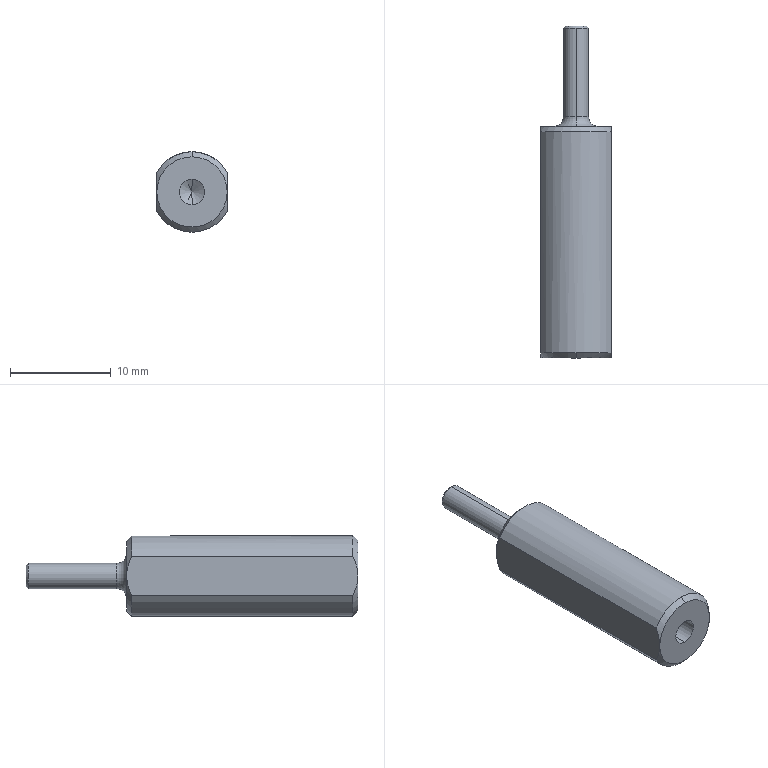Part | SolidWorks | features Chamfer 2, Fillet 1, HoleWzd 1, ICE 1, Revolution 1 | 1 solid | 24 faces | box 7 x 33 x 8 mm | volume 1085 mm3 | cone 10 | cylinder 7 | plane 5 | torus 2 | commonest cylinder face diameters 2.5 x4 8 x3
STEP:
#1=CARTESIAN_POINT('',(0.,33.,1.05));
#2=VERTEX_POINT('',#1);
#3=CARTESIAN_POINT('',(0.,33.,-1.05));
#4=VERTEX_POINT('',#3);
#5=CARTESIAN_POINT('',(0.,33.,0.));
#6=DIRECTION('',(0.,1.,0.));
#7=DIRECTION('',(0.,0.,1.));
#8=AXIS2_PLACEMENT_3D('',#5,#6,#7);
#9=CIRCLE('',#8,1.05);
#10=EDGE_CURVE('',#2,#4,#9,.T.);
#11=ORIENTED_EDGE('',*,*,#10,.F.);
#12=CARTESIAN_POINT('',(0.,32.8,1.25));
#13=VERTEX_POINT('',#12);
#14=CARTESIAN_POINT('',(0.,32.8,1.25));
#15=DIRECTION('',(0.,-0.7071,0.7071));
#16=VECTOR('',#15,1000.);
#17=LINE('',#14,#16);
#18=EDGE_CURVE('',#2,#13,#17,.T.);
#19=ORIENTED_EDGE('',*,*,#18,.T.);
#20=CARTESIAN_POINT('',(0.,32.8,-1.25));
#21=VERTEX_POINT('',#20);
#22=CARTESIAN_POINT('',(0.,32.8,0.));
#23=DIRECTION('',(0.,-1.,0.));
#24=DIRECTION('',(0.,0.,1.));
#25=AXIS2_PLACEMENT_3D('',#22,#23,#24);
#26=CIRCLE('',#25,1.25);
#27=EDGE_CURVE('',#21,#13,#26,.T.);
#28=ORIENTED_EDGE('',*,*,#27,.F.);
#29=CARTESIAN_POINT('',(0.,32.8,-1.25));
#30=DIRECTION('',(0.,-0.7071,-0.7071));
#31=VECTOR('',#30,1000.);
#32=LINE('',#29,#31);
#33=EDGE_CURVE('',#4,#21,#32,.T.);
#34=ORIENTED_EDGE('',*,*,#33,.F.);
#35=EDGE_LOOP('',(#11,#19,#28,#34));
#36=FACE_OUTER_BOUND('',#35,.T.);
#37=CARTESIAN_POINT('',(0.,32.8,0.));
#38=DIRECTION('',(0.,-1.,0.));
#39=DIRECTION('',(0.,0.,-1.));
#40=AXIS2_PLACEMENT_3D('',#37,#38,#39);
#41=CONICAL_SURFACE('',#40,1.25,0.7854);
#42=ADVANCED_FACE('',(#36),#41,.T.);
#43=CARTESIAN_POINT('',(0.,24.,-1.25));
#44=VERTEX_POINT('',#43);
#45=CARTESIAN_POINT('',(0.,24.,1.25));
#46=VERTEX_POINT('',#45);
#47=CARTESIAN_POINT('',(0.,24.,0.));
#48=DIRECTION('',(0.,1.,0.));
#49=DIRECTION('',(0.,0.,1.));
#50=AXIS2_PLACEMENT_3D('',#47,#48,#49);
#51=CIRCLE('',#50,1.25);
#52=EDGE_CURVE('',#44,#46,#51,.T.);
#53=ORIENTED_EDGE('',*,*,#52,.F.);
#54=CARTESIAN_POINT('',(0.,23.,-2.25));
#55=VERTEX_POINT('',#54);
#56=CARTESIAN_POINT('',(0.,24.,-2.25));
#57=DIRECTION('',(1.,0.,0.));
#58=DIRECTION('',(0.,0.,-1.));
#59=AXIS2_PLACEMENT_3D('',#56,#57,#58);
#60=CIRCLE('',#59,1.);
#61=EDGE_CURVE('',#44,#55,#60,.T.);
#62=ORIENTED_EDGE('',*,*,#61,.T.);
#63=CARTESIAN_POINT('',(0.,23.,2.25));
#64=VERTEX_POINT('',#63);
#65=CARTESIAN_POINT('',(0.,23.,0.));
#66=DIRECTION('',(0.,-1.,0.));
#67=DIRECTION('',(0.,0.,1.));
#68=AXIS2_PLACEMENT_3D('',#65,#66,#67);
#69=CIRCLE('',#68,2.25);
#70=EDGE_CURVE('',#64,#55,#69,.T.);
#71=ORIENTED_EDGE('',*,*,#70,.F.);
#72=CARTESIAN_POINT('',(0.,24.,2.25));
#73=DIRECTION('',(-1.,0.,0.));
#74=DIRECTION('',(0.,0.,1.));
#75=AXIS2_PLACEMENT_3D('',#72,#73,#74);
#76=CIRCLE('',#75,1.);
#77=EDGE_CURVE('',#46,#64,#76,.T.);
#78=ORIENTED_EDGE('',*,*,#77,.F.);
#79=EDGE_LOOP('',(#53,#62,#71,#78));
#80=FACE_OUTER_BOUND('',#79,.T.);
#81=CARTESIAN_POINT('',(0.,24.,0.));
#82=DIRECTION('',(0.,1.,0.));
#83=DIRECTION('',(0.,0.,1.));
#84=AXIS2_PLACEMENT_3D('',#81,#82,#83);
#85=TOROIDAL_SURFACE('',#84,2.25,1.);
#86=ADVANCED_FACE('',(#80),#85,.F.);
#87=CARTESIAN_POINT('',(0.,11.5,1.25));
#88=VERTEX_POINT('',#87);
#89=CARTESIAN_POINT('',(0.,11.5,-1.25));
#90=VERTEX_POINT('',#89);
#91=CARTESIAN_POINT('',(0.,11.5,0.));
#92=DIRECTION('',(0.,-1.,0.));
#93=DIRECTION('',(0.,0.,-1.));
#94=AXIS2_PLACEMENT_3D('',#91,#92,#93);
#95=CIRCLE('',#94,1.25);
#96=EDGE_CURVE('',#88,#90,#95,.T.);
#97=ORIENTED_EDGE('',*,*,#96,.F.);
#98=CARTESIAN_POINT('',(0.,0.,1.25));
#99=VERTEX_POINT('',#98);
#100=CARTESIAN_POINT('',(0.,0.,1.25));
#101=DIRECTION('',(0.,-1.,0.));
#102=VECTOR('',#101,1000.);
#103=LINE('',#100,#102);
#104=EDGE_CURVE('',#88,#99,#103,.T.);
#105=ORIENTED_EDGE('',*,*,#104,.T.);
#106=CARTESIAN_POINT('',(0.,0.,-1.25));
#107=VERTEX_POINT('',#106);
#108=CARTESIAN_POINT('',(0.,0.,0.));
#109=DIRECTION('',(0.,-1.,0.));
#110=DIRECTION('',(0.,0.,-1.));
#111=AXIS2_PLACEMENT_3D('',#108,#109,#110);
#112=CIRCLE('',#111,1.25);
#113=EDGE_CURVE('',#99,#107,#112,.T.);
#114=ORIENTED_EDGE('',*,*,#113,.T.);
#115=CARTESIAN_POINT('',(0.,0.,-1.25));
#116=DIRECTION('',(0.,-1.,0.));
#117=VECTOR('',#116,1000.);
#118=LINE('',#115,#117);
#119=EDGE_CURVE('',#90,#107,#118,.T.);
#120=ORIENTED_EDGE('',*,*,#119,.F.);
#121=EDGE_LOOP('',(#97,#105,#114,#120));
#122=FACE_OUTER_BOUND('',#121,.T.);
#123=CARTESIAN_POINT('',(0.,0.,0.));
#124=DIRECTION('',(0.,-1.,0.));
#125=DIRECTION('',(0.,0.,-1.));
#126=AXIS2_PLACEMENT_3D('',#123,#124,#125);
#127=CYLINDRICAL_SURFACE('',#126,1.25);
#128=ADVANCED_FACE('',(#122),#127,.F.);
#129=CARTESIAN_POINT('',(0.,12.251,0.));
#130=VERTEX_POINT('',#129);
#131=CARTESIAN_POINT('',(0.,11.5,-1.25));
#132=DIRECTION('',(0.,-0.515,-0.8572));
#133=VECTOR('',#132,1000.);
#134=LINE('',#131,#133);
#135=EDGE_CURVE('',#130,#90,#134,.T.);
#136=ORIENTED_EDGE('',*,*,#135,.F.);
#137=CARTESIAN_POINT('',(0.,11.5,1.25));
#138=DIRECTION('',(0.,-0.515,0.8572));
#139=VECTOR('',#138,1000.);
#140=LINE('',#137,#139);
#141=EDGE_CURVE('',#130,#88,#140,.T.);
#142=ORIENTED_EDGE('',*,*,#141,.T.);
#143=ORIENTED_EDGE('',*,*,#96,.T.);
#144=EDGE_LOOP('',(#136,#142,#143));
#145=FACE_OUTER_BOUND('',#144,.T.);
#146=CARTESIAN_POINT('',(0.,11.5,0.));
#147=DIRECTION('',(0.,-1.,0.));
#148=DIRECTION('',(0.,0.,-1.));
#149=AXIS2_PLACEMENT_3D('',#146,#147,#148);
#150=CONICAL_SURFACE('',#149,1.25,1.03);
#151=ADVANCED_FACE('',(#145),#150,.F.);
#152=CARTESIAN_POINT('',(-3.5,22.5,-1.936));
#153=VERTEX_POINT('',#152);
#154=CARTESIAN_POINT('',(0.,22.5,-4.));
#155=VERTEX_POINT('',#154);
#156=CARTESIAN_POINT('',(0.,22.5,0.));
#157=DIRECTION('',(0.,-1.,0.));
#158=DIRECTION('',(0.,0.,1.));
#159=AXIS2_PLACEMENT_3D('',#156,#157,#158);
#160=CIRCLE('',#159,4.);
#161=EDGE_CURVE('',#153,#155,#160,.T.);
#162=ORIENTED_EDGE('',*,*,#161,.T.);
#163=CARTESIAN_POINT('',(0.,0.5,-4.));
#164=VERTEX_POINT('',#163);
#165=CARTESIAN_POINT('',(0.,-0.5244,-4.));
#166=DIRECTION('',(0.,-1.,0.));
#167=VECTOR('',#166,1000.);
#168=LINE('',#165,#167);
#169=EDGE_CURVE('',#155,#164,#168,.T.);
#170=ORIENTED_EDGE('',*,*,#169,.T.);
#171=CARTESIAN_POINT('',(-3.5,0.5,-1.936));
#172=VERTEX_POINT('',#171);
#173=CARTESIAN_POINT('',(0.,0.5,0.));
#174=DIRECTION('',(0.,1.,0.));
#175=DIRECTION('',(0.,0.,-1.));
#176=AXIS2_PLACEMENT_3D('',#173,#174,#175);
#177=CIRCLE('',#176,4.);
#178=EDGE_CURVE('',#164,#172,#177,.T.);
#179=ORIENTED_EDGE('',*,*,#178,.T.);
#180=CARTESIAN_POINT('',(-3.5,-0.5244,-1.936));
#181=DIRECTION('',(0.,-1.,0.));
#182=VECTOR('',#181,1000.);
#183=LINE('',#180,#182);
#184=EDGE_CURVE('',#153,#172,#183,.T.);
#185=ORIENTED_EDGE('',*,*,#184,.F.);
#186=EDGE_LOOP('',(#162,#170,#179,#185));
#187=FACE_OUTER_BOUND('',#186,.T.);
#188=CARTESIAN_POINT('',(0.,-0.5244,0.));
#189=DIRECTION('',(0.,-1.,0.));
#190=DIRECTION('',(0.,0.,-1.));
#191=AXIS2_PLACEMENT_3D('',#188,#189,#190);
#192=CYLINDRICAL_SURFACE('',#191,4.);
#193=ADVANCED_FACE('',(#187),#192,.T.);
#194=ORIENTED_EDGE('',*,*,#27,.T.);
#195=CARTESIAN_POINT('',(0.,-0.5244,1.25));
#196=DIRECTION('',(0.,-1.,0.));
#197=VECTOR('',#196,1000.);
#198=LINE('',#195,#197);
#199=EDGE_CURVE('',#13,#46,#198,.T.);
#200=ORIENTED_EDGE('',*,*,#199,.T.);
#201=CARTESIAN_POINT('',(0.,24.,0.));
#202=DIRECTION('',(0.,1.,0.));
#203=DIRECTION('',(0.,0.,1.));
#204=AXIS2_PLACEMENT_3D('',#201,#202,#203);
#205=CIRCLE('',#204,1.25);
#206=EDGE_CURVE('',#46,#44,#205,.T.);
#207=ORIENTED_EDGE('',*,*,#206,.T.);
#208=CARTESIAN_POINT('',(0.,-0.5244,-1.25));
#209=DIRECTION('',(0.,-1.,0.));
#210=VECTOR('',#209,1000.);
#211=LINE('',#208,#210);
#212=EDGE_CURVE('',#21,#44,#211,.T.);
#213=ORIENTED_EDGE('',*,*,#212,.F.);
#214=EDGE_LOOP('',(#194,#200,#207,#213));
#215=FACE_OUTER_BOUND('',#214,.T.);
#216=CARTESIAN_POINT('',(0.,-0.5244,0.));
#217=DIRECTION('',(0.,-1.,0.));
#218=DIRECTION('',(0.,0.,-1.));
#219=AXIS2_PLACEMENT_3D('',#216,#217,#218);
#220=CYLINDRICAL_SURFACE('',#219,1.25);
#221=ADVANCED_FACE('',(#215),#220,.T.);
#222=CARTESIAN_POINT('',(0.,23.,-3.5));
#223=VERTEX_POINT('',#222);
#224=CARTESIAN_POINT('',(-3.5,23.,0.));
#225=VERTEX_POINT('',#224);
#226=CARTESIAN_POINT('',(0.,23.,0.));
#227=DIRECTION('',(0.,1.,0.));
#228=DIRECTION('',(0.,0.,1.));
#229=AXIS2_PLACEMENT_3D('',#226,#227,#228);
#230=CIRCLE('',#229,3.5);
#231=EDGE_CURVE('',#223,#225,#230,.T.);
#232=ORIENTED_EDGE('',*,*,#231,.F.);
#233=CARTESIAN_POINT('',(0.,22.5,-4.));
#234=DIRECTION('',(0.,-0.7071,-0.7071));
#235=VECTOR('',#234,1000.);
#236=LINE('',#233,#235);
#237=EDGE_CURVE('',#223,#155,#236,.T.);
#238=ORIENTED_EDGE('',*,*,#237,.T.);
#239=ORIENTED_EDGE('',*,*,#161,.F.);
#240=CARTESIAN_POINT('',(-3.5,23.,0.));
#241=CARTESIAN_POINT('',(-3.5,23.,-0.34));
#242=CARTESIAN_POINT('',(-3.5,22.95,-0.673));
#243=CARTESIAN_POINT('',(-3.5,22.77,-1.328));
#244=CARTESIAN_POINT('',(-3.5,22.645,-1.638));
#245=CARTESIAN_POINT('',(-3.5,22.5,-1.936));
#246=B_SPLINE_CURVE_WITH_KNOTS('',3,(#240,#241,#242,#243,#244,#245),.UNSPECIFIED.,.F.,.F.,(4,2,4),(0.004182,0.005183,0.006184),.UNSPECIFIED.);
#247=EDGE_CURVE('',#225,#153,#246,.T.);
#248=ORIENTED_EDGE('',*,*,#247,.F.);
#249=EDGE_LOOP('',(#232,#238,#239,#248));
#250=FACE_OUTER_BOUND('',#249,.T.);
#251=CARTESIAN_POINT('',(0.,22.5,0.));
#252=DIRECTION('',(0.,-1.,0.));
#253=DIRECTION('',(0.,0.,-1.));
#254=AXIS2_PLACEMENT_3D('',#251,#252,#253);
#255=CONICAL_SURFACE('',#254,4.,0.7854);
#256=ADVANCED_FACE('',(#250),#255,.T.);
#257=CARTESIAN_POINT('',(0.,0.,3.5));
#258=VERTEX_POINT('',#257);
#259=CARTESIAN_POINT('',(-3.5,0.,0.));
#260=VERTEX_POINT('',#259);
#261=CARTESIAN_POINT('',(0.,0.,0.));
#262=DIRECTION('',(0.,-1.,0.));
#263=DIRECTION('',(0.,0.,-1.));
#264=AXIS2_PLACEMENT_3D('',#261,#262,#263);
#265=CIRCLE('',#264,3.5);
#266=EDGE_CURVE('',#258,#260,#265,.T.);
#267=ORIENTED_EDGE('',*,*,#266,.F.);
#268=CARTESIAN_POINT('',(0.,0.5,4.));
#269=VERTEX_POINT('',#268);
#270=CARTESIAN_POINT('',(0.,0.,3.5));
#271=DIRECTION('',(0.,0.7071,0.7071));
#272=VECTOR('',#271,1000.);
#273=LINE('',#270,#272);
#274=EDGE_CURVE('',#258,#269,#273,.T.);
#275=ORIENTED_EDGE('',*,*,#274,.T.);
#276=CARTESIAN_POINT('',(-3.5,0.5,1.936));
#277=VERTEX_POINT('',#276);
#278=CARTESIAN_POINT('',(0.,0.5,0.));
#279=DIRECTION('',(0.,1.,0.));
#280=DIRECTION('',(0.,0.,-1.));
#281=AXIS2_PLACEMENT_3D('',#278,#279,#280);
#282=CIRCLE('',#281,4.);
#283=EDGE_CURVE('',#277,#269,#282,.T.);
#284=ORIENTED_EDGE('',*,*,#283,.F.);
#285=CARTESIAN_POINT('',(-3.5,0.,0.));
#286=CARTESIAN_POINT('',(-3.5,0.,0.3393));
#287=CARTESIAN_POINT('',(-3.5,0.05023,0.6719));
#288=CARTESIAN_POINT('',(-3.5,0.1834,1.158));
#289=CARTESIAN_POINT('',(-3.5,0.2376,1.319));
#290=CARTESIAN_POINT('',(-3.5,0.3596,1.633));
#291=CARTESIAN_POINT('',(-3.5,0.4273,1.786));
#292=CARTESIAN_POINT('',(-3.5,0.5,1.936));
#293=B_SPLINE_CURVE_WITH_KNOTS('',3,(#285,#286,#287,#288,#289,#290,#291,#292),.UNSPECIFIED.,.F.,.F.,(4,2,2,4),(0.01206,0.01306,0.01356,0.01406),.UNSPECIFIED.);
#294=EDGE_CURVE('',#260,#277,#293,.T.);
#295=ORIENTED_EDGE('',*,*,#294,.F.);
#296=EDGE_LOOP('',(#267,#275,#284,#295));
#297=FACE_OUTER_BOUND('',#296,.T.);
#298=CARTESIAN_POINT('',(0.,0.,0.));
#299=DIRECTION('',(0.,1.,0.));
#300=DIRECTION('',(0.,0.,1.));
#301=AXIS2_PLACEMENT_3D('',#298,#299,#300);
#302=CONICAL_SURFACE('',#301,3.5,0.7854);
#303=ADVANCED_FACE('',(#297),#302,.T.);
#304=CARTESIAN_POINT('',(3.5,22.5,1.936));
#305=VERTEX_POINT('',#304);
#306=CARTESIAN_POINT('',(3.5,0.5,1.936));
#307=VERTEX_POINT('',#306);
#308=CARTESIAN_POINT('',(3.5,-0.5244,1.936));
#309=DIRECTION('',(0.,-1.,0.));
#310=VECTOR('',#309,1000.);
#311=LINE('',#308,#310);
#312=EDGE_CURVE('',#305,#307,#311,.T.);
#313=ORIENTED_EDGE('',*,*,#312,.F.);
#314=CARTESIAN_POINT('',(-3.5,22.5,1.936));
#315=VERTEX_POINT('',#314);
#316=CARTESIAN_POINT('',(0.,22.5,0.));
#317=DIRECTION('',(0.,-1.,0.));
#318=DIRECTION('',(0.,0.,1.));
#319=AXIS2_PLACEMENT_3D('',#316,#317,#318);
#320=CIRCLE('',#319,4.);
#321=EDGE_CURVE('',#305,#315,#320,.T.);
#322=ORIENTED_EDGE('',*,*,#321,.T.);
#323=CARTESIAN_POINT('',(-3.5,-0.5244,1.936));
#324=DIRECTION('',(0.,1.,0.));
#325=VECTOR('',#324,1000.);
#326=LINE('',#323,#325);
#327=EDGE_CURVE('',#277,#315,#326,.T.);
#328=ORIENTED_EDGE('',*,*,#327,.F.);
#329=ORIENTED_EDGE('',*,*,#283,.T.);
#330=CARTESIAN_POINT('',(0.,0.5,0.));
#331=DIRECTION('',(0.,1.,0.));
#332=DIRECTION('',(0.,0.,-1.));
#333=AXIS2_PLACEMENT_3D('',#330,#331,#332);
#334=CIRCLE('',#333,4.);
#335=EDGE_CURVE('',#269,#307,#334,.T.);
#336=ORIENTED_EDGE('',*,*,#335,.T.);
#337=EDGE_LOOP('',(#313,#322,#328,#329,#336));
#338=FACE_OUTER_BOUND('',#337,.T.);
#339=CARTESIAN_POINT('',(0.,-0.5244,0.));
#340=DIRECTION('',(0.,-1.,0.));
#341=DIRECTION('',(0.,0.,-1.));
#342=AXIS2_PLACEMENT_3D('',#339,#340,#341);
#343=CYLINDRICAL_SURFACE('',#342,4.);
#344=ADVANCED_FACE('',(#338),#343,.T.);
#345=ORIENTED_EDGE('',*,*,#274,.F.);
#346=CARTESIAN_POINT('',(3.5,0.,0.));
#347=VERTEX_POINT('',#346);
#348=CARTESIAN_POINT('',(0.,0.,0.));
#349=DIRECTION('',(0.,-1.,0.));
#350=DIRECTION('',(0.,0.,-1.));
#351=AXIS2_PLACEMENT_3D('',#348,#349,#350);
#352=CIRCLE('',#351,3.5);
#353=EDGE_CURVE('',#347,#258,#352,.T.);
#354=ORIENTED_EDGE('',*,*,#353,.F.);
#355=CARTESIAN_POINT('',(3.5,0.5,1.936));
#356=CARTESIAN_POINT('',(3.5,0.4273,1.786));
#357=CARTESIAN_POINT('',(3.5,0.3596,1.633));
#358=CARTESIAN_POINT('',(3.5,0.2376,1.319));
#359=CARTESIAN_POINT('',(3.5,0.1834,1.158));
#360=CARTESIAN_POINT('',(3.5,0.05023,0.6719));
#361=CARTESIAN_POINT('',(3.5,0.,0.3393));
#362=CARTESIAN_POINT('',(3.5,0.,0.));
#363=B_SPLINE_CURVE_WITH_KNOTS('',3,(#355,#356,#357,#358,#359,#360,#361,#362),.UNSPECIFIED.,.F.,.F.,(4,2,2,4),(0.002184,0.002684,0.003183,0.004182),.UNSPECIFIED.);
#364=EDGE_CURVE('',#307,#347,#363,.T.);
#365=ORIENTED_EDGE('',*,*,#364,.F.);
#366=ORIENTED_EDGE('',*,*,#335,.F.);
#367=EDGE_LOOP('',(#345,#354,#365,#366));
#368=FACE_OUTER_BOUND('',#367,.T.);
#369=CARTESIAN_POINT('',(0.,0.,0.));
#370=DIRECTION('',(0.,1.,0.));
#371=DIRECTION('',(0.,0.,1.));
#372=AXIS2_PLACEMENT_3D('',#369,#370,#371);
#373=CONICAL_SURFACE('',#372,3.5,0.7854);
#374=ADVANCED_FACE('',(#368),#373,.T.);
#375=ORIENTED_EDGE('',*,*,#237,.F.);
#376=CARTESIAN_POINT('',(3.5,23.,0.));
#377=VERTEX_POINT('',#376);
#378=CARTESIAN_POINT('',(0.,23.,0.));
#379=DIRECTION('',(0.,1.,0.));
#380=DIRECTION('',(0.,0.,1.));
#381=AXIS2_PLACEMENT_3D('',#378,#379,#380);
#382=CIRCLE('',#381,3.5);
#383=EDGE_CURVE('',#377,#223,#382,.T.);
#384=ORIENTED_EDGE('',*,*,#383,.F.);
#385=CARTESIAN_POINT('',(3.5,22.5,-1.936));
#386=VERTEX_POINT('',#385);
#387=CARTESIAN_POINT('',(3.5,22.5,-1.936));
#388=CARTESIAN_POINT('',(3.5,22.645,-1.638));
#389=CARTESIAN_POINT('',(3.5,22.77,-1.328));
#390=CARTESIAN_POINT('',(3.5,22.95,-0.673));
#391=CARTESIAN_POINT('',(3.5,23.,-0.34));
#392=CARTESIAN_POINT('',(3.5,23.,0.));
#393=B_SPLINE_CURVE_WITH_KNOTS('',3,(#387,#388,#389,#390,#391,#392),.UNSPECIFIED.,.F.,.F.,(4,2,4),(0.01007,0.01107,0.01206),.UNSPECIFIED.);
#394=EDGE_CURVE('',#386,#377,#393,.T.);
#395=ORIENTED_EDGE('',*,*,#394,.F.);
#396=CARTESIAN_POINT('',(0.,22.5,0.));
#397=DIRECTION('',(0.,-1.,0.));
#398=DIRECTION('',(0.,0.,1.));
#399=AXIS2_PLACEMENT_3D('',#396,#397,#398);
#400=CIRCLE('',#399,4.);
#401=EDGE_CURVE('',#155,#386,#400,.T.);
#402=ORIENTED_EDGE('',*,*,#401,.F.);
#403=EDGE_LOOP('',(#375,#384,#395,#402));
#404=FACE_OUTER_BOUND('',#403,.T.);
#405=CARTESIAN_POINT('',(0.,22.5,0.));
#406=DIRECTION('',(0.,-1.,0.));
#407=DIRECTION('',(0.,0.,-1.));
#408=AXIS2_PLACEMENT_3D('',#405,#406,#407);
#409=CONICAL_SURFACE('',#408,4.,0.7854);
#410=ADVANCED_FACE('',(#404),#409,.T.);
#411=CARTESIAN_POINT('',(0.,33.,0.));
#412=DIRECTION('',(0.,1.,0.));
#413=DIRECTION('',(0.,0.,1.));
#414=AXIS2_PLACEMENT_3D('',#411,#412,#413);
#415=CIRCLE('',#414,1.05);
#416=EDGE_CURVE('',#4,#2,#415,.T.);
#417=ORIENTED_EDGE('',*,*,#416,.T.);
#418=ORIENTED_EDGE('',*,*,#10,.T.);
#419=EDGE_LOOP('',(#417,#418));
#420=FACE_OUTER_BOUND('',#419,.T.);
#421=CARTESIAN_POINT('',(0.,33.,0.));
#422=DIRECTION('',(0.,1.,0.));
#423=DIRECTION('',(0.,0.,1.));
#424=AXIS2_PLACEMENT_3D('',#421,#422,#423);
#425=PLANE('',#424);
#426=ADVANCED_FACE('',(#420),#425,.T.);
#427=ORIENTED_EDGE('',*,*,#199,.F.);
#428=CARTESIAN_POINT('',(0.,32.8,0.));
#429=DIRECTION('',(0.,-1.,0.));
#430=DIRECTION('',(0.,0.,1.));
#431=AXIS2_PLACEMENT_3D('',#428,#429,#430);
#432=CIRCLE('',#431,1.25);
#433=EDGE_CURVE('',#13,#21,#432,.T.);
#434=ORIENTED_EDGE('',*,*,#433,.T.);
#435=ORIENTED_EDGE('',*,*,#212,.T.);
#436=ORIENTED_EDGE('',*,*,#52,.T.);
#437=EDGE_LOOP('',(#427,#434,#435,#436));
#438=FACE_OUTER_BOUND('',#437,.T.);
#439=CARTESIAN_POINT('',(0.,-0.5244,0.));
#440=DIRECTION('',(0.,-1.,0.));
#441=DIRECTION('',(0.,0.,-1.));
#442=AXIS2_PLACEMENT_3D('',#439,#440,#441);
#443=CYLINDRICAL_SURFACE('',#442,1.25);
#444=ADVANCED_FACE('',(#438),#443,.T.);
#445=ORIENTED_EDGE('',*,*,#70,.T.);
#446=CARTESIAN_POINT('',(0.,23.,0.));
#447=DIRECTION('',(0.,-1.,0.));
#448=DIRECTION('',(0.,0.,1.));
#449=AXIS2_PLACEMENT_3D('',#446,#447,#448);
#450=CIRCLE('',#449,2.25);
#451=EDGE_CURVE('',#55,#64,#450,.T.);
#452=ORIENTED_EDGE('',*,*,#451,.T.);
#453=EDGE_LOOP('',(#445,#452));
#454=FACE_BOUND('',#453,.T.);
#455=ORIENTED_EDGE('',*,*,#383,.T.);
#456=ORIENTED_EDGE('',*,*,#231,.T.);
#457=CARTESIAN_POINT('',(0.,23.,0.));
#458=DIRECTION('',(0.,1.,0.));
#459=DIRECTION('',(0.,0.,1.));
#460=AXIS2_PLACEMENT_3D('',#457,#458,#459);
#461=CIRCLE('',#460,3.5);
#462=EDGE_CURVE('',#225,#377,#461,.T.);
#463=ORIENTED_EDGE('',*,*,#462,.T.);
#464=EDGE_LOOP('',(#455,#456,#463));
#465=FACE_OUTER_BOUND('',#464,.T.);
#466=CARTESIAN_POINT('',(1.25,23.,0.));
#467=DIRECTION('',(0.,1.,0.));
#468=DIRECTION('',(0.,0.,1.));
#469=AXIS2_PLACEMENT_3D('',#466,#467,#468);
#470=PLANE('',#469);
#471=ADVANCED_FACE('',(#454,#465),#470,.T.);
#472=ORIENTED_EDGE('',*,*,#169,.F.);
#473=ORIENTED_EDGE('',*,*,#401,.T.);
#474=CARTESIAN_POINT('',(3.5,0.5,-1.936));
#475=VERTEX_POINT('',#474);
#476=CARTESIAN_POINT('',(3.5,-0.5244,-1.936));
#477=DIRECTION('',(0.,1.,0.));
#478=VECTOR('',#477,1000.);
#479=LINE('',#476,#478);
#480=EDGE_CURVE('',#475,#386,#479,.T.);
#481=ORIENTED_EDGE('',*,*,#480,.F.);
#482=CARTESIAN_POINT('',(0.,0.5,0.));
#483=DIRECTION('',(0.,1.,0.));
#484=DIRECTION('',(0.,0.,-1.));
#485=AXIS2_PLACEMENT_3D('',#482,#483,#484);
#486=CIRCLE('',#485,4.);
#487=EDGE_CURVE('',#475,#164,#486,.T.);
#488=ORIENTED_EDGE('',*,*,#487,.T.);
#489=EDGE_LOOP('',(#472,#473,#481,#488));
#490=FACE_OUTER_BOUND('',#489,.T.);
#491=CARTESIAN_POINT('',(0.,-0.5244,0.));
#492=DIRECTION('',(0.,-1.,0.));
#493=DIRECTION('',(0.,0.,-1.));
#494=AXIS2_PLACEMENT_3D('',#491,#492,#493);
#495=CYLINDRICAL_SURFACE('',#494,4.);
#496=ADVANCED_FACE('',(#490),#495,.T.);
#497=ORIENTED_EDGE('',*,*,#353,.T.);
#498=ORIENTED_EDGE('',*,*,#266,.T.);
#499=CARTESIAN_POINT('',(0.,0.,0.));
#500=DIRECTION('',(0.,-1.,0.));
#501=DIRECTION('',(0.,0.,-1.));
#502=AXIS2_PLACEMENT_3D('',#499,#500,#501);
#503=CIRCLE('',#502,3.5);
#504=EDGE_CURVE('',#260,#347,#503,.T.);
#505=ORIENTED_EDGE('',*,*,#504,.T.);
#506=EDGE_LOOP('',(#497,#498,#505));
#507=FACE_OUTER_BOUND('',#506,.T.);
#508=CARTESIAN_POINT('',(0.,0.,0.));
#509=DIRECTION('',(0.,-1.,0.));
#510=DIRECTION('',(0.,0.,-1.));
#511=AXIS2_PLACEMENT_3D('',#508,#509,#510);
#512=CIRCLE('',#511,1.25);
#513=EDGE_CURVE('',#107,#99,#512,.T.);
#514=ORIENTED_EDGE('',*,*,#513,.F.);
#515=ORIENTED_EDGE('',*,*,#113,.F.);
#516=EDGE_LOOP('',(#514,#515));
#517=FACE_BOUND('',#516,.T.);
#518=CARTESIAN_POINT('',(0.,0.,0.));
#519=DIRECTION('',(0.,-1.,0.));
#520=DIRECTION('',(0.,0.,-1.));
#521=AXIS2_PLACEMENT_3D('',#518,#519,#520);
#522=PLANE('',#521);
#523=ADVANCED_FACE('',(#507,#517),#522,.T.);
#524=ORIENTED_EDGE('',*,*,#141,.F.);
#525=ORIENTED_EDGE('',*,*,#135,.T.);
#526=CARTESIAN_POINT('',(0.,11.5,0.));
#527=DIRECTION('',(0.,-1.,0.));
#528=DIRECTION('',(0.,0.,-1.));
#529=AXIS2_PLACEMENT_3D('',#526,#527,#528);
#530=CIRCLE('',#529,1.25);
#531=EDGE_CURVE('',#90,#88,#530,.T.);
#532=ORIENTED_EDGE('',*,*,#531,.T.);
#533=EDGE_LOOP('',(#524,#525,#532));
#534=FACE_OUTER_BOUND('',#533,.T.);
#535=CARTESIAN_POINT('',(0.,11.5,0.));
#536=DIRECTION('',(0.,-1.,0.));
#537=DIRECTION('',(0.,0.,-1.));
#538=AXIS2_PLACEMENT_3D('',#535,#536,#537);
#539=CONICAL_SURFACE('',#538,1.25,1.03);
#540=ADVANCED_FACE('',(#534),#539,.F.);
#541=ORIENTED_EDGE('',*,*,#104,.F.);
#542=ORIENTED_EDGE('',*,*,#531,.F.);
#543=ORIENTED_EDGE('',*,*,#119,.T.);
#544=ORIENTED_EDGE('',*,*,#513,.T.);
#545=EDGE_LOOP('',(#541,#542,#543,#544));
#546=FACE_OUTER_BOUND('',#545,.T.);
#547=CARTESIAN_POINT('',(0.,0.,0.));
#548=DIRECTION('',(0.,-1.,0.));
#549=DIRECTION('',(0.,0.,-1.));
#550=AXIS2_PLACEMENT_3D('',#547,#548,#549);
#551=CYLINDRICAL_SURFACE('',#550,1.25);
#552=ADVANCED_FACE('',(#546),#551,.F.);
#553=CARTESIAN_POINT('',(3.5,0.,0.));
#554=CARTESIAN_POINT('',(3.5,0.,-0.34));
#555=CARTESIAN_POINT('',(3.5,0.05018,-0.673));
#556=CARTESIAN_POINT('',(3.5,0.2302,-1.328));
#557=CARTESIAN_POINT('',(3.5,0.3555,-1.638));
#558=CARTESIAN_POINT('',(3.5,0.5,-1.936));
#559=B_SPLINE_CURVE_WITH_KNOTS('',3,(#553,#554,#555,#556,#557,#558),.UNSPECIFIED.,.F.,.F.,(4,2,4),(0.004182,0.005183,0.006184),.UNSPECIFIED.);
#560=EDGE_CURVE('',#347,#475,#559,.T.);
#561=ORIENTED_EDGE('',*,*,#560,.F.);
#562=ORIENTED_EDGE('',*,*,#504,.F.);
#563=CARTESIAN_POINT('',(-3.5,0.5,-1.936));
#564=CARTESIAN_POINT('',(-3.5,0.3555,-1.638));
#565=CARTESIAN_POINT('',(-3.5,0.2302,-1.328));
#566=CARTESIAN_POINT('',(-3.5,0.05018,-0.673));
#567=CARTESIAN_POINT('',(-3.5,0.,-0.34));
#568=CARTESIAN_POINT('',(-3.5,0.,0.));
#569=B_SPLINE_CURVE_WITH_KNOTS('',3,(#563,#564,#565,#566,#567,#568),.UNSPECIFIED.,.F.,.F.,(4,2,4),(0.01007,0.01107,0.01206),.UNSPECIFIED.);
#570=EDGE_CURVE('',#172,#260,#569,.T.);
#571=ORIENTED_EDGE('',*,*,#570,.F.);
#572=ORIENTED_EDGE('',*,*,#178,.F.);
#573=ORIENTED_EDGE('',*,*,#487,.F.);
#574=EDGE_LOOP('',(#561,#562,#571,#572,#573));
#575=FACE_OUTER_BOUND('',#574,.T.);
#576=CARTESIAN_POINT('',(0.,0.,0.));
#577=DIRECTION('',(0.,1.,0.));
#578=DIRECTION('',(0.,0.,1.));
#579=AXIS2_PLACEMENT_3D('',#576,#577,#578);
#580=CONICAL_SURFACE('',#579,3.5,0.7854);
#581=ADVANCED_FACE('',(#575),#580,.T.);
#582=CARTESIAN_POINT('',(3.5,23.,0.));
#583=CARTESIAN_POINT('',(3.5,23.,0.3393));
#584=CARTESIAN_POINT('',(3.5,22.95,0.6719));
#585=CARTESIAN_POINT('',(3.5,22.817,1.158));
#586=CARTESIAN_POINT('',(3.5,22.762,1.319));
#587=CARTESIAN_POINT('',(3.5,22.64,1.633));
#588=CARTESIAN_POINT('',(3.5,22.573,1.786));
#589=CARTESIAN_POINT('',(3.5,22.5,1.936));
#590=B_SPLINE_CURVE_WITH_KNOTS('',3,(#582,#583,#584,#585,#586,#587,#588,#589),.UNSPECIFIED.,.F.,.F.,(4,2,2,4),(0.01206,0.01306,0.01356,0.01406),.UNSPECIFIED.);
#591=EDGE_CURVE('',#377,#305,#590,.T.);
#592=ORIENTED_EDGE('',*,*,#591,.F.);
#593=ORIENTED_EDGE('',*,*,#462,.F.);
#594=CARTESIAN_POINT('',(-3.5,22.5,1.936));
#595=CARTESIAN_POINT('',(-3.5,22.573,1.786));
#596=CARTESIAN_POINT('',(-3.5,22.64,1.633));
#597=CARTESIAN_POINT('',(-3.5,22.762,1.319));
#598=CARTESIAN_POINT('',(-3.5,22.817,1.158));
#599=CARTESIAN_POINT('',(-3.5,22.95,0.6719));
#600=CARTESIAN_POINT('',(-3.5,23.,0.3393));
#601=CARTESIAN_POINT('',(-3.5,23.,0.));
#602=B_SPLINE_CURVE_WITH_KNOTS('',3,(#594,#595,#596,#597,#598,#599,#600,#601),.UNSPECIFIED.,.F.,.F.,(4,2,2,4),(0.002184,0.002684,0.003183,0.004182),.UNSPECIFIED.);
#603=EDGE_CURVE('',#315,#225,#602,.T.);
#604=ORIENTED_EDGE('',*,*,#603,.F.);
#605=ORIENTED_EDGE('',*,*,#321,.F.);
#606=EDGE_LOOP('',(#592,#593,#604,#605));
#607=FACE_OUTER_BOUND('',#606,.T.);
#608=CARTESIAN_POINT('',(0.,22.5,0.));
#609=DIRECTION('',(0.,-1.,0.));
#610=DIRECTION('',(0.,0.,-1.));
#611=AXIS2_PLACEMENT_3D('',#608,#609,#610);
#612=CONICAL_SURFACE('',#611,4.,0.7854);
#613=ADVANCED_FACE('',(#607),#612,.T.);
#614=ORIENTED_EDGE('',*,*,#61,.F.);
#615=ORIENTED_EDGE('',*,*,#206,.F.);
#616=ORIENTED_EDGE('',*,*,#77,.T.);
#617=ORIENTED_EDGE('',*,*,#451,.F.);
#618=EDGE_LOOP('',(#614,#615,#616,#617));
#619=FACE_OUTER_BOUND('',#618,.T.);
#620=CARTESIAN_POINT('',(0.,24.,0.));
#621=DIRECTION('',(0.,1.,0.));
#622=DIRECTION('',(0.,0.,1.));
#623=AXIS2_PLACEMENT_3D('',#620,#621,#622);
#624=TOROIDAL_SURFACE('',#623,2.25,1.);
#625=ADVANCED_FACE('',(#619),#624,.F.);
#626=ORIENTED_EDGE('',*,*,#570,.T.);
#627=ORIENTED_EDGE('',*,*,#294,.T.);
#628=ORIENTED_EDGE('',*,*,#327,.T.);
#629=ORIENTED_EDGE('',*,*,#603,.T.);
#630=ORIENTED_EDGE('',*,*,#247,.T.);
#631=ORIENTED_EDGE('',*,*,#184,.T.);
#632=EDGE_LOOP('',(#626,#627,#628,#629,#630,#631));
#633=FACE_OUTER_BOUND('',#632,.T.);
#634=CARTESIAN_POINT('',(-3.5,23.,-5.));
#635=DIRECTION('',(1.,0.,0.));
#636=DIRECTION('',(0.,1.,0.));
#637=AXIS2_PLACEMENT_3D('',#634,#635,#636);
#638=PLANE('',#637);
#639=ADVANCED_FACE('',(#633),#638,.F.);
#640=ORIENTED_EDGE('',*,*,#364,.T.);
#641=ORIENTED_EDGE('',*,*,#560,.T.);
#642=ORIENTED_EDGE('',*,*,#480,.T.);
#643=ORIENTED_EDGE('',*,*,#394,.T.);
#644=ORIENTED_EDGE('',*,*,#591,.T.);
#645=ORIENTED_EDGE('',*,*,#312,.T.);
#646=EDGE_LOOP('',(#640,#641,#642,#643,#644,#645));
#647=FACE_OUTER_BOUND('',#646,.T.);
#648=CARTESIAN_POINT('',(3.5,23.,-5.));
#649=DIRECTION('',(-1.,0.,0.));
#650=DIRECTION('',(0.,-1.,0.));
#651=AXIS2_PLACEMENT_3D('',#648,#649,#650);
#652=PLANE('',#651);
#653=ADVANCED_FACE('',(#647),#652,.F.);
#654=ORIENTED_EDGE('',*,*,#18,.F.);
#655=ORIENTED_EDGE('',*,*,#416,.F.);
#656=ORIENTED_EDGE('',*,*,#33,.T.);
#657=ORIENTED_EDGE('',*,*,#433,.F.);
#658=EDGE_LOOP('',(#654,#655,#656,#657));
#659=FACE_OUTER_BOUND('',#658,.T.);
#660=CARTESIAN_POINT('',(0.,32.8,0.));
#661=DIRECTION('',(0.,-1.,0.));
#662=DIRECTION('',(0.,0.,-1.));
#663=AXIS2_PLACEMENT_3D('',#660,#661,#662);
#664=CONICAL_SURFACE('',#663,1.25,0.7854);
#665=ADVANCED_FACE('',(#659),#664,.T.);
#666=CLOSED_SHELL('',(#42,#86,#128,#151,#193,#221,#256,#303,#344,#374,#410,#426,#444,#471,#496,#523,#540,#552,#581,#613,#625,#639,#653,#665));
#667=MANIFOLD_SOLID_BREP('',#666);
#668=CARTESIAN_POINT('',(0.,0.,0.));
#669=DIRECTION('',(0.,0.,1.));
#670=DIRECTION('',(1.,0.,0.));
#671=AXIS2_PLACEMENT_3D('',#668,#669,#670);
#672=(LENGTH_UNIT()NAMED_UNIT(*)SI_UNIT(.MILLI.,.METRE.));
#673=UNCERTAINTY_MEASURE_WITH_UNIT(LENGTH_MEASURE(0.00001),#672,'','');
#674=(NAMED_UNIT(*)PLANE_ANGLE_UNIT()SI_UNIT($,.RADIAN.));
#675=(NAMED_UNIT(*)SI_UNIT($,.STERADIAN.)SOLID_ANGLE_UNIT());
#676=(GEOMETRIC_REPRESENTATION_CONTEXT(3)GLOBAL_UNCERTAINTY_ASSIGNED_CONTEXT((#673))GLOBAL_UNIT_ASSIGNED_CONTEXT((#672,#674,#675))REPRESENTATION_CONTEXT('',''));
#677=ADVANCED_BREP_SHAPE_REPRESENTATION('',(#667,#671),#676);